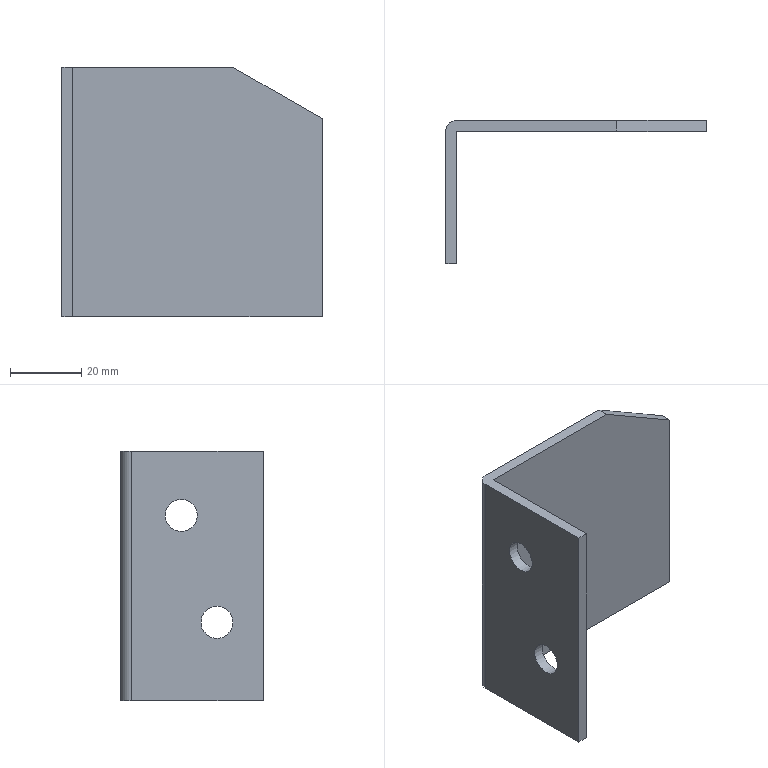Part | STEP file | lll_id4138_x_t | 1 solid | 12 faces | box 73 x 40 x 70 mm | volume 22040 mm3 | plane 9 | cylinder 3 | commonest cylinder face diameters 9 x2 6 x1
STEP:
#1=CARTESIAN_POINT('',(3970.435,402.5,-253.5));
#2=VERTEX_POINT('',#1);
#3=CARTESIAN_POINT('',(3970.435,402.5,-258.));
#4=DIRECTION('',(-1.,0.,0.));
#5=DIRECTION('',(0.,0.,1.));
#6=AXIS2_PLACEMENT_3D('',#3,#4,#5);
#7=CIRCLE('',#6,4.5);
#8=EDGE_CURVE('',#2,#2,#7,.T.);
#9=ORIENTED_EDGE('',*,*,#8,.T.);
#10=EDGE_LOOP('',(#9));
#11=FACE_BOUND('',#10,.T.);
#12=CARTESIAN_POINT('',(3970.435,412.5,-223.5));
#13=VERTEX_POINT('',#12);
#14=CARTESIAN_POINT('',(3970.435,412.5,-228.));
#15=DIRECTION('',(-1.,0.,0.));
#16=DIRECTION('',(0.,0.,1.));
#17=AXIS2_PLACEMENT_3D('',#14,#15,#16);
#18=CIRCLE('',#17,4.5);
#19=EDGE_CURVE('',#13,#13,#18,.T.);
#20=ORIENTED_EDGE('',*,*,#19,.T.);
#21=EDGE_LOOP('',(#20));
#22=FACE_BOUND('',#21,.T.);
#23=CARTESIAN_POINT('',(3970.435,426.5,-210.));
#24=VERTEX_POINT('',#23);
#25=CARTESIAN_POINT('',(3970.435,426.5,-280.));
#26=VERTEX_POINT('',#25);
#27=CARTESIAN_POINT('',(3970.435,426.5,-160.8));
#28=DIRECTION('',(0.,0.,-1.));
#29=VECTOR('',#28,1.);
#30=LINE('',#27,#29);
#31=EDGE_CURVE('',#24,#26,#30,.T.);
#32=ORIENTED_EDGE('',*,*,#31,.F.);
#33=CARTESIAN_POINT('',(3970.435,389.5,-210.));
#34=VERTEX_POINT('',#33);
#35=CARTESIAN_POINT('',(3970.435,340.5,-210.));
#36=DIRECTION('',(0.,1.,0.));
#37=VECTOR('',#36,1.);
#38=LINE('',#35,#37);
#39=EDGE_CURVE('',#34,#24,#38,.T.);
#40=ORIENTED_EDGE('',*,*,#39,.F.);
#41=CARTESIAN_POINT('',(3970.435,389.5,-280.));
#42=VERTEX_POINT('',#41);
#43=CARTESIAN_POINT('',(3970.435,389.5,-214.281));
#44=DIRECTION('',(0.,0.,-1.));
#45=VECTOR('',#44,1.);
#46=LINE('',#43,#45);
#47=EDGE_CURVE('',#34,#42,#46,.T.);
#48=ORIENTED_EDGE('',*,*,#47,.T.);
#49=CARTESIAN_POINT('',(3970.435,340.5,-280.));
#50=DIRECTION('',(0.,1.,0.));
#51=VECTOR('',#50,1.);
#52=LINE('',#49,#51);
#53=EDGE_CURVE('',#42,#26,#52,.T.);
#54=ORIENTED_EDGE('',*,*,#53,.T.);
#55=EDGE_LOOP('',(#32,#40,#48,#54));
#56=FACE_BOUND('',#55,.T.);
#57=CARTESIAN_POINT('',(3970.435,340.5,-214.281));
#58=DIRECTION('',(-1.,0.,0.));
#59=DIRECTION('',(0.,0.,-1.));
#60=AXIS2_PLACEMENT_3D('',#57,#58,#59);
#61=PLANE('',#60);
#62=ADVANCED_FACE('',(#11,#22,#56),#61,.F.);
#63=CARTESIAN_POINT('',(3967.435,412.5,-232.5));
#64=VERTEX_POINT('',#63);
#65=CARTESIAN_POINT('',(3967.435,412.5,-228.));
#66=DIRECTION('',(-1.,0.,0.));
#67=DIRECTION('',(0.,0.,-1.));
#68=AXIS2_PLACEMENT_3D('',#65,#66,#67);
#69=CIRCLE('',#68,4.5);
#70=EDGE_CURVE('',#64,#64,#69,.T.);
#71=ORIENTED_EDGE('',*,*,#70,.T.);
#72=EDGE_LOOP('',(#71));
#73=FACE_BOUND('',#72,.T.);
#74=ORIENTED_EDGE('',*,*,#19,.F.);
#75=EDGE_LOOP('',(#74));
#76=FACE_BOUND('',#75,.T.);
#77=CARTESIAN_POINT('',(3967.435,412.5,-228.));
#78=DIRECTION('',(-1.,0.,0.));
#79=DIRECTION('',(0.,1.,0.));
#80=AXIS2_PLACEMENT_3D('',#77,#78,#79);
#81=CYLINDRICAL_SURFACE('',#80,4.5);
#82=ADVANCED_FACE('',(#73,#76),#81,.F.);
#83=ORIENTED_EDGE('',*,*,#47,.F.);
#84=CARTESIAN_POINT('',(3967.435,389.5,-210.));
#85=VERTEX_POINT('',#84);
#86=CARTESIAN_POINT('',(3986.964,389.5,-210.));
#87=DIRECTION('',(1.,0.,0.));
#88=VECTOR('',#87,1.);
#89=LINE('',#86,#88);
#90=EDGE_CURVE('',#85,#34,#89,.T.);
#91=ORIENTED_EDGE('',*,*,#90,.F.);
#92=CARTESIAN_POINT('',(3967.435,389.5,-280.));
#93=VERTEX_POINT('',#92);
#94=CARTESIAN_POINT('',(3967.435,389.5,-214.281));
#95=DIRECTION('',(0.,0.,-1.));
#96=VECTOR('',#95,1.);
#97=LINE('',#94,#96);
#98=EDGE_CURVE('',#85,#93,#97,.T.);
#99=ORIENTED_EDGE('',*,*,#98,.T.);
#100=CARTESIAN_POINT('',(3967.435,389.5,-280.));
#101=DIRECTION('',(-1.,0.,0.));
#102=VECTOR('',#101,1.);
#103=LINE('',#100,#102);
#104=EDGE_CURVE('',#42,#93,#103,.T.);
#105=ORIENTED_EDGE('',*,*,#104,.F.);
#106=EDGE_LOOP('',(#83,#91,#99,#105));
#107=FACE_OUTER_BOUND('',#106,.T.);
#108=CARTESIAN_POINT('',(3986.964,389.5,-224.151));
#109=DIRECTION('',(0.,1.,0.));
#110=DIRECTION('',(0.5,0.,0.866));
#111=AXIS2_PLACEMENT_3D('',#108,#109,#110);
#112=PLANE('',#111);
#113=ADVANCED_FACE('',(#107),#112,.F.);
#114=CARTESIAN_POINT('',(4015.397,426.5,-210.));
#115=VERTEX_POINT('',#114);
#116=CARTESIAN_POINT('',(4015.397,429.5,-210.));
#117=VERTEX_POINT('',#116);
#118=CARTESIAN_POINT('',(4015.397,1424.5,-210.));
#119=DIRECTION('',(0.,1.,0.));
#120=VECTOR('',#119,1.);
#121=LINE('',#118,#120);
#122=EDGE_CURVE('',#115,#117,#121,.T.);
#123=ORIENTED_EDGE('',*,*,#122,.T.);
#124=CARTESIAN_POINT('',(3970.435,429.5,-210.));
#125=VERTEX_POINT('',#124);
#126=CARTESIAN_POINT('',(3162.435,429.5,-210.));
#127=DIRECTION('',(1.,0.,0.));
#128=VECTOR('',#127,1.);
#129=LINE('',#126,#128);
#130=EDGE_CURVE('',#125,#117,#129,.T.);
#131=ORIENTED_EDGE('',*,*,#130,.F.);
#132=CARTESIAN_POINT('',(3967.435,426.5,-210.));
#133=VERTEX_POINT('',#132);
#134=CARTESIAN_POINT('',(3970.435,426.5,-210.));
#135=DIRECTION('',(0.,0.,1.));
#136=DIRECTION('',(1.,0.,0.));
#137=AXIS2_PLACEMENT_3D('',#134,#135,#136);
#138=CIRCLE('',#137,3.);
#139=EDGE_CURVE('',#125,#133,#138,.T.);
#140=ORIENTED_EDGE('',*,*,#139,.T.);
#141=CARTESIAN_POINT('',(3967.435,482.821,-210.));
#142=DIRECTION('',(0.,-1.,0.));
#143=VECTOR('',#142,1.);
#144=LINE('',#141,#143);
#145=EDGE_CURVE('',#133,#85,#144,.T.);
#146=ORIENTED_EDGE('',*,*,#145,.T.);
#147=ORIENTED_EDGE('',*,*,#90,.T.);
#148=ORIENTED_EDGE('',*,*,#39,.T.);
#149=CARTESIAN_POINT('',(4020.435,426.5,-210.));
#150=DIRECTION('',(-1.,0.,0.));
#151=VECTOR('',#150,1.);
#152=LINE('',#149,#151);
#153=EDGE_CURVE('',#115,#24,#152,.T.);
#154=ORIENTED_EDGE('',*,*,#153,.F.);
#155=EDGE_LOOP('',(#123,#131,#140,#146,#147,#148,#154));
#156=FACE_OUTER_BOUND('',#155,.T.);
#157=CARTESIAN_POINT('',(3162.435,482.821,-210.));
#158=DIRECTION('',(0.,0.,1.));
#159=DIRECTION('',(1.,0.,0.));
#160=AXIS2_PLACEMENT_3D('',#157,#158,#159);
#161=PLANE('',#160);
#162=ADVANCED_FACE('',(#156),#161,.T.);
#163=CARTESIAN_POINT('',(3967.435,402.5,-253.5));
#164=VERTEX_POINT('',#163);
#165=CARTESIAN_POINT('',(3967.435,402.5,-258.));
#166=DIRECTION('',(1.,0.,0.));
#167=DIRECTION('',(0.,0.,1.));
#168=AXIS2_PLACEMENT_3D('',#165,#166,#167);
#169=CIRCLE('',#168,4.5);
#170=EDGE_CURVE('',#164,#164,#169,.T.);
#171=ORIENTED_EDGE('',*,*,#170,.T.);
#172=EDGE_LOOP('',(#171));
#173=FACE_BOUND('',#172,.T.);
#174=ORIENTED_EDGE('',*,*,#145,.F.);
#175=CARTESIAN_POINT('',(3967.435,426.5,-280.));
#176=VERTEX_POINT('',#175);
#177=CARTESIAN_POINT('',(3967.435,426.5,-250.));
#178=DIRECTION('',(0.,0.,-1.));
#179=VECTOR('',#178,1.);
#180=LINE('',#177,#179);
#181=EDGE_CURVE('',#133,#176,#180,.T.);
#182=ORIENTED_EDGE('',*,*,#181,.T.);
#183=CARTESIAN_POINT('',(3967.435,165.5,-280.));
#184=DIRECTION('',(0.,1.,0.));
#185=VECTOR('',#184,1.);
#186=LINE('',#183,#185);
#187=EDGE_CURVE('',#93,#176,#186,.T.);
#188=ORIENTED_EDGE('',*,*,#187,.F.);
#189=ORIENTED_EDGE('',*,*,#98,.F.);
#190=EDGE_LOOP('',(#174,#182,#188,#189));
#191=FACE_BOUND('',#190,.T.);
#192=ORIENTED_EDGE('',*,*,#70,.F.);
#193=EDGE_LOOP('',(#192));
#194=FACE_BOUND('',#193,.T.);
#195=CARTESIAN_POINT('',(3967.435,340.5,-214.281));
#196=DIRECTION('',(-1.,0.,0.));
#197=DIRECTION('',(0.,0.,-1.));
#198=AXIS2_PLACEMENT_3D('',#195,#196,#197);
#199=PLANE('',#198);
#200=ADVANCED_FACE('',(#173,#191,#194),#199,.T.);
#201=ORIENTED_EDGE('',*,*,#187,.T.);
#202=CARTESIAN_POINT('',(3970.435,429.5,-280.));
#203=VERTEX_POINT('',#202);
#204=CARTESIAN_POINT('',(3970.435,426.5,-280.));
#205=DIRECTION('',(0.,0.,-1.));
#206=DIRECTION('',(-1.,0.,0.));
#207=AXIS2_PLACEMENT_3D('',#204,#205,#206);
#208=CIRCLE('',#207,3.);
#209=EDGE_CURVE('',#176,#203,#208,.T.);
#210=ORIENTED_EDGE('',*,*,#209,.T.);
#211=CARTESIAN_POINT('',(4040.435,429.5,-280.));
#212=VERTEX_POINT('',#211);
#213=CARTESIAN_POINT('',(3967.435,429.5,-280.));
#214=DIRECTION('',(-1.,0.,0.));
#215=VECTOR('',#214,1.);
#216=LINE('',#213,#215);
#217=EDGE_CURVE('',#212,#203,#216,.T.);
#218=ORIENTED_EDGE('',*,*,#217,.F.);
#219=CARTESIAN_POINT('',(4040.435,426.5,-280.));
#220=VERTEX_POINT('',#219);
#221=CARTESIAN_POINT('',(4040.435,789.821,-280.));
#222=DIRECTION('',(0.,1.,0.));
#223=VECTOR('',#222,1.);
#224=LINE('',#221,#223);
#225=EDGE_CURVE('',#220,#212,#224,.T.);
#226=ORIENTED_EDGE('',*,*,#225,.F.);
#227=CARTESIAN_POINT('',(4020.435,426.5,-280.));
#228=DIRECTION('',(-1.,0.,0.));
#229=VECTOR('',#228,1.);
#230=LINE('',#227,#229);
#231=EDGE_CURVE('',#220,#26,#230,.T.);
#232=ORIENTED_EDGE('',*,*,#231,.T.);
#233=ORIENTED_EDGE('',*,*,#53,.F.);
#234=ORIENTED_EDGE('',*,*,#104,.T.);
#235=EDGE_LOOP('',(#201,#210,#218,#226,#232,#233,#234));
#236=FACE_OUTER_BOUND('',#235,.T.);
#237=CARTESIAN_POINT('',(3967.435,165.5,-280.));
#238=DIRECTION('',(0.,0.,-1.));
#239=DIRECTION('',(0.,1.,0.));
#240=AXIS2_PLACEMENT_3D('',#237,#238,#239);
#241=PLANE('',#240);
#242=ADVANCED_FACE('',(#236),#241,.T.);
#243=ORIENTED_EDGE('',*,*,#130,.T.);
#244=CARTESIAN_POINT('',(4040.435,429.5,-224.456));
#245=VERTEX_POINT('',#244);
#246=CARTESIAN_POINT('',(3966.435,429.5,-181.732));
#247=DIRECTION('',(-0.866,0.,0.5));
#248=VECTOR('',#247,1.);
#249=LINE('',#246,#248);
#250=EDGE_CURVE('',#245,#117,#249,.T.);
#251=ORIENTED_EDGE('',*,*,#250,.F.);
#252=CARTESIAN_POINT('',(4040.435,429.5,-160.8));
#253=DIRECTION('',(0.,0.,1.));
#254=VECTOR('',#253,1.);
#255=LINE('',#252,#254);
#256=EDGE_CURVE('',#212,#245,#255,.T.);
#257=ORIENTED_EDGE('',*,*,#256,.F.);
#258=ORIENTED_EDGE('',*,*,#217,.T.);
#259=CARTESIAN_POINT('',(3970.435,429.5,-210.));
#260=DIRECTION('',(0.,0.,1.));
#261=VECTOR('',#260,1.);
#262=LINE('',#259,#261);
#263=EDGE_CURVE('',#203,#125,#262,.T.);
#264=ORIENTED_EDGE('',*,*,#263,.T.);
#265=EDGE_LOOP('',(#243,#251,#257,#258,#264));
#266=FACE_OUTER_BOUND('',#265,.T.);
#267=CARTESIAN_POINT('',(3968.935,429.5,-236.917));
#268=DIRECTION('',(0.,-1.,0.));
#269=DIRECTION('',(1.,0.,0.));
#270=AXIS2_PLACEMENT_3D('',#267,#268,#269);
#271=PLANE('',#270);
#272=ADVANCED_FACE('',(#266),#271,.F.);
#273=CARTESIAN_POINT('',(4040.435,426.5,-224.456));
#274=VERTEX_POINT('',#273);
#275=CARTESIAN_POINT('',(4040.435,426.5,-160.8));
#276=DIRECTION('',(0.,0.,-1.));
#277=VECTOR('',#276,1.);
#278=LINE('',#275,#277);
#279=EDGE_CURVE('',#274,#220,#278,.T.);
#280=ORIENTED_EDGE('',*,*,#279,.F.);
#281=CARTESIAN_POINT('',(4019.176,426.5,-212.182));
#282=DIRECTION('',(-0.866,0.,0.5));
#283=VECTOR('',#282,1.);
#284=LINE('',#281,#283);
#285=EDGE_CURVE('',#274,#115,#284,.T.);
#286=ORIENTED_EDGE('',*,*,#285,.T.);
#287=ORIENTED_EDGE('',*,*,#153,.T.);
#288=ORIENTED_EDGE('',*,*,#31,.T.);
#289=ORIENTED_EDGE('',*,*,#231,.F.);
#290=EDGE_LOOP('',(#280,#286,#287,#288,#289));
#291=FACE_OUTER_BOUND('',#290,.T.);
#292=CARTESIAN_POINT('',(4020.435,426.5,-210.));
#293=DIRECTION('',(0.,1.,0.));
#294=DIRECTION('',(0.,0.,1.));
#295=AXIS2_PLACEMENT_3D('',#292,#293,#294);
#296=PLANE('',#295);
#297=ADVANCED_FACE('',(#291),#296,.F.);
#298=ORIENTED_EDGE('',*,*,#256,.T.);
#299=CARTESIAN_POINT('',(4040.435,789.821,-224.456));
#300=DIRECTION('',(0.,-1.,0.));
#301=VECTOR('',#300,1.);
#302=LINE('',#299,#301);
#303=EDGE_CURVE('',#245,#274,#302,.T.);
#304=ORIENTED_EDGE('',*,*,#303,.T.);
#305=ORIENTED_EDGE('',*,*,#279,.T.);
#306=ORIENTED_EDGE('',*,*,#225,.T.);
#307=EDGE_LOOP('',(#298,#304,#305,#306));
#308=FACE_OUTER_BOUND('',#307,.T.);
#309=CARTESIAN_POINT('',(4040.435,789.821,-160.8));
#310=DIRECTION('',(-1.,0.,0.));
#311=DIRECTION('',(0.,0.,1.));
#312=AXIS2_PLACEMENT_3D('',#309,#310,#311);
#313=PLANE('',#312);
#314=ADVANCED_FACE('',(#308),#313,.F.);
#315=ORIENTED_EDGE('',*,*,#139,.F.);
#316=ORIENTED_EDGE('',*,*,#263,.F.);
#317=ORIENTED_EDGE('',*,*,#209,.F.);
#318=ORIENTED_EDGE('',*,*,#181,.F.);
#319=EDGE_LOOP('',(#315,#316,#317,#318));
#320=FACE_OUTER_BOUND('',#319,.T.);
#321=CARTESIAN_POINT('',(3970.435,426.5,-214.281));
#322=DIRECTION('',(0.,0.,1.));
#323=DIRECTION('',(1.,0.,0.));
#324=AXIS2_PLACEMENT_3D('',#321,#322,#323);
#325=CYLINDRICAL_SURFACE('',#324,3.);
#326=ADVANCED_FACE('',(#320),#325,.T.);
#327=ORIENTED_EDGE('',*,*,#170,.F.);
#328=EDGE_LOOP('',(#327));
#329=FACE_BOUND('',#328,.T.);
#330=ORIENTED_EDGE('',*,*,#8,.F.);
#331=EDGE_LOOP('',(#330));
#332=FACE_BOUND('',#331,.T.);
#333=CARTESIAN_POINT('',(3967.435,402.5,-258.));
#334=DIRECTION('',(-1.,0.,0.));
#335=DIRECTION('',(0.,1.,0.));
#336=AXIS2_PLACEMENT_3D('',#333,#334,#335);
#337=CYLINDRICAL_SURFACE('',#336,4.5);
#338=ADVANCED_FACE('',(#329,#332),#337,.F.);
#339=ORIENTED_EDGE('',*,*,#122,.F.);
#340=ORIENTED_EDGE('',*,*,#285,.F.);
#341=ORIENTED_EDGE('',*,*,#303,.F.);
#342=ORIENTED_EDGE('',*,*,#250,.T.);
#343=EDGE_LOOP('',(#339,#340,#341,#342));
#344=FACE_OUTER_BOUND('',#343,.T.);
#345=CARTESIAN_POINT('',(3966.435,1424.5,-181.732));
#346=DIRECTION('',(0.5,0.,0.866));
#347=DIRECTION('',(0.866,0.,-0.5));
#348=AXIS2_PLACEMENT_3D('',#345,#346,#347);
#349=PLANE('',#348);
#350=ADVANCED_FACE('',(#344),#349,.T.);
#351=CLOSED_SHELL('',(#62,#82,#113,#162,#200,#242,#272,#297,#314,#326,#338,#350));
#352=MANIFOLD_SOLID_BREP('',#351);
#353=(LENGTH_UNIT()NAMED_UNIT(*)SI_UNIT(.MILLI.,.METRE.));
#354=UNCERTAINTY_MEASURE_WITH_UNIT(LENGTH_MEASURE(0.00002),#353,'','');
#355=(NAMED_UNIT(*)PLANE_ANGLE_UNIT()SI_UNIT($,.RADIAN.));
#356=PLANE_ANGLE_MEASURE_WITH_UNIT(PLANE_ANGLE_MEASURE(0.01745),#355);
#357=DIMENSIONAL_EXPONENTS(0.,0.,0.,0.,0.,0.,0.);
#358=(CONVERSION_BASED_UNIT('DEGREE',#356)NAMED_UNIT(#357)PLANE_ANGLE_UNIT());
#359=(NAMED_UNIT(*)SI_UNIT($,.STERADIAN.)SOLID_ANGLE_UNIT());
#360=(GEOMETRIC_REPRESENTATION_CONTEXT(3)GLOBAL_UNCERTAINTY_ASSIGNED_CONTEXT((#354))GLOBAL_UNIT_ASSIGNED_CONTEXT((#353,#358,#359))REPRESENTATION_CONTEXT('',''));
#361=ADVANCED_BREP_SHAPE_REPRESENTATION('',(#352),#360);